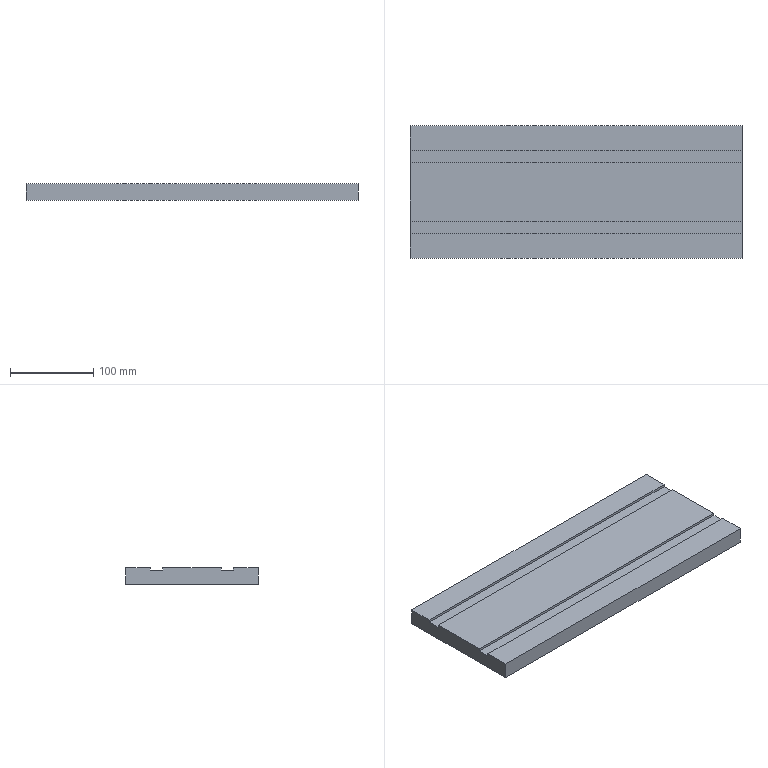Part | STEP file | Tube feed_id638_x_t | 1 solid | 14 faces | box 400 x 160 x 20 mm | volume 1244000 mm3 | plane 14
STEP:
#1=CARTESIAN_POINT('',(0.,0.,0.));
#2=DIRECTION('',(0.,0.,1.));
#3=DIRECTION('',(1.,0.,0.));
#4=AXIS2_PLACEMENT_3D('',#1,#2,#3);
#5=CARTESIAN_POINT('',(66.,461.936,-199.));
#6=VERTEX_POINT('',#5);
#7=CARTESIAN_POINT('',(66.,461.936,-202.));
#8=VERTEX_POINT('',#7);
#9=CARTESIAN_POINT('',(66.,461.936,-199.819));
#10=DIRECTION('',(0.,0.,-1.));
#11=VECTOR('',#10,1.);
#12=LINE('',#9,#11);
#13=CARTESIAN_POINT('',(66.,491.936,-199.));
#14=DIRECTION('',(1.,0.,0.));
#15=DIRECTION('',(0.,1.,0.));
#16=AXIS2_PLACEMENT_3D('',#13,#14,#15);
#17=PLANE('',#16);
#18=CARTESIAN_POINT('',(-30.,-0.8185));
#19=DIRECTION('',(0.,-1.));
#20=VECTOR('',#19,1.);
#21=LINE('',#18,#20);
#22=(GEOMETRIC_REPRESENTATION_CONTEXT(2)PARAMETRIC_REPRESENTATION_CONTEXT()REPRESENTATION_CONTEXT('',''));
#23=DEFINITIONAL_REPRESENTATION('',(#21),#22);
#24=PCURVE('',#17,#23);
#25=CARTESIAN_POINT('',(1137.73,461.936,-199.819));
#26=DIRECTION('',(0.,1.,0.));
#27=DIRECTION('',(0.,0.,1.));
#28=AXIS2_PLACEMENT_3D('',#25,#26,#27);
#29=PLANE('',#28);
#30=CARTESIAN_POINT('',(0.,-1071.73));
#31=DIRECTION('',(-1.,0.));
#32=VECTOR('',#31,1.);
#33=LINE('',#30,#32);
#34=(GEOMETRIC_REPRESENTATION_CONTEXT(2)PARAMETRIC_REPRESENTATION_CONTEXT()REPRESENTATION_CONTEXT('',''));
#35=DEFINITIONAL_REPRESENTATION('',(#33),#34);
#36=PCURVE('',#29,#35);
#37=SURFACE_CURVE('',#12,(#24,#36),.PCURVE_S1.);
#38=EDGE_CURVE('',#6,#8,#37,.T.);
#39=ORIENTED_EDGE('',*,*,#38,.F.);
#40=CARTESIAN_POINT('',(66.,491.936,-199.));
#41=VERTEX_POINT('',#40);
#42=CARTESIAN_POINT('',(66.,491.936,-199.));
#43=DIRECTION('',(0.,-1.,0.));
#44=VECTOR('',#43,1.);
#45=LINE('',#42,#44);
#46=CARTESIAN_POINT('',(0.,0.));
#47=DIRECTION('',(-1.,0.));
#48=VECTOR('',#47,1.);
#49=LINE('',#46,#48);
#50=(GEOMETRIC_REPRESENTATION_CONTEXT(2)PARAMETRIC_REPRESENTATION_CONTEXT()REPRESENTATION_CONTEXT('',''));
#51=DEFINITIONAL_REPRESENTATION('',(#49),#50);
#52=PCURVE('',#17,#51);
#53=CARTESIAN_POINT('',(0.,0.,-199.));
#54=DIRECTION('',(0.,0.,1.));
#55=DIRECTION('',(1.,0.,0.));
#56=AXIS2_PLACEMENT_3D('',#53,#54,#55);
#57=PLANE('',#56);
#58=CARTESIAN_POINT('',(66.,491.936));
#59=DIRECTION('',(0.,-1.));
#60=VECTOR('',#59,1.);
#61=LINE('',#58,#60);
#62=(GEOMETRIC_REPRESENTATION_CONTEXT(2)PARAMETRIC_REPRESENTATION_CONTEXT()REPRESENTATION_CONTEXT('',''));
#63=DEFINITIONAL_REPRESENTATION('',(#61),#62);
#64=PCURVE('',#57,#63);
#65=SURFACE_CURVE('',#45,(#52,#64),.PCURVE_S1.);
#66=EDGE_CURVE('',#41,#6,#65,.T.);
#67=ORIENTED_EDGE('',*,*,#66,.F.);
#68=CARTESIAN_POINT('',(66.,491.936,-219.));
#69=VERTEX_POINT('',#68);
#70=CARTESIAN_POINT('',(66.,491.936,-199.));
#71=DIRECTION('',(0.,0.,-1.));
#72=VECTOR('',#71,1.);
#73=LINE('',#70,#72);
#74=CARTESIAN_POINT('',(0.,0.));
#75=DIRECTION('',(0.,-1.));
#76=VECTOR('',#75,1.);
#77=LINE('',#74,#76);
#78=(GEOMETRIC_REPRESENTATION_CONTEXT(2)PARAMETRIC_REPRESENTATION_CONTEXT()REPRESENTATION_CONTEXT('',''));
#79=DEFINITIONAL_REPRESENTATION('',(#77),#78);
#80=PCURVE('',#17,#79);
#81=CARTESIAN_POINT('',(466.,491.936,-199.));
#82=DIRECTION('',(0.,-1.,0.));
#83=DIRECTION('',(0.,0.,-1.));
#84=AXIS2_PLACEMENT_3D('',#81,#82,#83);
#85=PLANE('',#84);
#86=CARTESIAN_POINT('',(0.,-400.));
#87=DIRECTION('',(1.,0.));
#88=VECTOR('',#87,1.);
#89=LINE('',#86,#88);
#90=(GEOMETRIC_REPRESENTATION_CONTEXT(2)PARAMETRIC_REPRESENTATION_CONTEXT()REPRESENTATION_CONTEXT('',''));
#91=DEFINITIONAL_REPRESENTATION('',(#89),#90);
#92=PCURVE('',#85,#91);
#93=SURFACE_CURVE('',#73,(#80,#92),.PCURVE_S1.);
#94=EDGE_CURVE('',#41,#69,#93,.T.);
#95=ORIENTED_EDGE('',*,*,#94,.T.);
#96=CARTESIAN_POINT('',(66.,331.936,-219.));
#97=VERTEX_POINT('',#96);
#98=CARTESIAN_POINT('',(66.,491.936,-219.));
#99=DIRECTION('',(0.,-1.,0.));
#100=VECTOR('',#99,1.);
#101=LINE('',#98,#100);
#102=CARTESIAN_POINT('',(0.,-20.));
#103=DIRECTION('',(-1.,0.));
#104=VECTOR('',#103,1.);
#105=LINE('',#102,#104);
#106=(GEOMETRIC_REPRESENTATION_CONTEXT(2)PARAMETRIC_REPRESENTATION_CONTEXT()REPRESENTATION_CONTEXT('',''));
#107=DEFINITIONAL_REPRESENTATION('',(#105),#106);
#108=PCURVE('',#17,#107);
#109=CARTESIAN_POINT('',(0.,0.,-219.));
#110=DIRECTION('',(0.,0.,1.));
#111=DIRECTION('',(1.,0.,0.));
#112=AXIS2_PLACEMENT_3D('',#109,#110,#111);
#113=PLANE('',#112);
#114=CARTESIAN_POINT('',(66.,491.936));
#115=DIRECTION('',(0.,-1.));
#116=VECTOR('',#115,1.);
#117=LINE('',#114,#116);
#118=(GEOMETRIC_REPRESENTATION_CONTEXT(2)PARAMETRIC_REPRESENTATION_CONTEXT()REPRESENTATION_CONTEXT('',''));
#119=DEFINITIONAL_REPRESENTATION('',(#117),#118);
#120=PCURVE('',#113,#119);
#121=SURFACE_CURVE('',#101,(#108,#120),.PCURVE_S1.);
#122=EDGE_CURVE('',#69,#97,#121,.T.);
#123=ORIENTED_EDGE('',*,*,#122,.T.);
#124=CARTESIAN_POINT('',(66.,331.936,-199.));
#125=VERTEX_POINT('',#124);
#126=CARTESIAN_POINT('',(66.,331.936,-199.));
#127=DIRECTION('',(0.,0.,-1.));
#128=VECTOR('',#127,1.);
#129=LINE('',#126,#128);
#130=CARTESIAN_POINT('',(-160.,0.));
#131=DIRECTION('',(0.,-1.));
#132=VECTOR('',#131,1.);
#133=LINE('',#130,#132);
#134=(GEOMETRIC_REPRESENTATION_CONTEXT(2)PARAMETRIC_REPRESENTATION_CONTEXT()REPRESENTATION_CONTEXT('',''));
#135=DEFINITIONAL_REPRESENTATION('',(#133),#134);
#136=PCURVE('',#17,#135);
#137=CARTESIAN_POINT('',(66.,331.936,-199.));
#138=DIRECTION('',(0.,1.,0.));
#139=DIRECTION('',(-1.,0.,0.));
#140=AXIS2_PLACEMENT_3D('',#137,#138,#139);
#141=PLANE('',#140);
#142=CARTESIAN_POINT('',(0.,0.));
#143=DIRECTION('',(0.,-1.));
#144=VECTOR('',#143,1.);
#145=LINE('',#142,#144);
#146=(GEOMETRIC_REPRESENTATION_CONTEXT(2)PARAMETRIC_REPRESENTATION_CONTEXT()REPRESENTATION_CONTEXT('',''));
#147=DEFINITIONAL_REPRESENTATION('',(#145),#146);
#148=PCURVE('',#141,#147);
#149=SURFACE_CURVE('',#129,(#136,#148),.PCURVE_S1.);
#150=EDGE_CURVE('',#125,#97,#149,.T.);
#151=ORIENTED_EDGE('',*,*,#150,.F.);
#152=CARTESIAN_POINT('',(66.,361.936,-199.));
#153=VERTEX_POINT('',#152);
#154=CARTESIAN_POINT('',(66.,491.936,-199.));
#155=DIRECTION('',(0.,-1.,0.));
#156=VECTOR('',#155,1.);
#157=LINE('',#154,#156);
#158=CARTESIAN_POINT('',(0.,0.));
#159=DIRECTION('',(-1.,0.));
#160=VECTOR('',#159,1.);
#161=LINE('',#158,#160);
#162=(GEOMETRIC_REPRESENTATION_CONTEXT(2)PARAMETRIC_REPRESENTATION_CONTEXT()REPRESENTATION_CONTEXT('',''));
#163=DEFINITIONAL_REPRESENTATION('',(#161),#162);
#164=PCURVE('',#17,#163);
#165=CARTESIAN_POINT('',(0.,0.,-199.));
#166=DIRECTION('',(0.,0.,1.));
#167=DIRECTION('',(1.,0.,0.));
#168=AXIS2_PLACEMENT_3D('',#165,#166,#167);
#169=PLANE('',#168);
#170=CARTESIAN_POINT('',(66.,491.936));
#171=DIRECTION('',(0.,-1.));
#172=VECTOR('',#171,1.);
#173=LINE('',#170,#172);
#174=(GEOMETRIC_REPRESENTATION_CONTEXT(2)PARAMETRIC_REPRESENTATION_CONTEXT()REPRESENTATION_CONTEXT('',''));
#175=DEFINITIONAL_REPRESENTATION('',(#173),#174);
#176=PCURVE('',#169,#175);
#177=SURFACE_CURVE('',#157,(#164,#176),.PCURVE_S1.);
#178=EDGE_CURVE('',#153,#125,#177,.T.);
#179=ORIENTED_EDGE('',*,*,#178,.F.);
#180=CARTESIAN_POINT('',(66.,361.936,-202.));
#181=VERTEX_POINT('',#180);
#182=CARTESIAN_POINT('',(66.,361.936,-201.));
#183=DIRECTION('',(0.,0.,1.));
#184=VECTOR('',#183,1.);
#185=LINE('',#182,#184);
#186=CARTESIAN_POINT('',(-130.,-2.));
#187=DIRECTION('',(0.,1.));
#188=VECTOR('',#187,1.);
#189=LINE('',#186,#188);
#190=(GEOMETRIC_REPRESENTATION_CONTEXT(2)PARAMETRIC_REPRESENTATION_CONTEXT()REPRESENTATION_CONTEXT('',''));
#191=DEFINITIONAL_REPRESENTATION('',(#189),#190);
#192=PCURVE('',#17,#191);
#193=CARTESIAN_POINT('',(1137.73,361.936,-201.));
#194=DIRECTION('',(0.,-1.,0.));
#195=DIRECTION('',(0.,0.,-1.));
#196=AXIS2_PLACEMENT_3D('',#193,#194,#195);
#197=PLANE('',#196);
#198=CARTESIAN_POINT('',(0.,-1071.73));
#199=DIRECTION('',(-1.,0.));
#200=VECTOR('',#199,1.);
#201=LINE('',#198,#200);
#202=(GEOMETRIC_REPRESENTATION_CONTEXT(2)PARAMETRIC_REPRESENTATION_CONTEXT()REPRESENTATION_CONTEXT('',''));
#203=DEFINITIONAL_REPRESENTATION('',(#201),#202);
#204=PCURVE('',#197,#203);
#205=SURFACE_CURVE('',#185,(#192,#204),.PCURVE_S1.);
#206=EDGE_CURVE('',#181,#153,#205,.T.);
#207=ORIENTED_EDGE('',*,*,#206,.F.);
#208=CARTESIAN_POINT('',(66.,376.936,-202.));
#209=VERTEX_POINT('',#208);
#210=CARTESIAN_POINT('',(66.,376.936,-202.));
#211=DIRECTION('',(0.,-1.,0.));
#212=VECTOR('',#211,1.);
#213=LINE('',#210,#212);
#214=CARTESIAN_POINT('',(-115.,-3.));
#215=DIRECTION('',(-1.,0.));
#216=VECTOR('',#215,1.);
#217=LINE('',#214,#216);
#218=(GEOMETRIC_REPRESENTATION_CONTEXT(2)PARAMETRIC_REPRESENTATION_CONTEXT()REPRESENTATION_CONTEXT('',''));
#219=DEFINITIONAL_REPRESENTATION('',(#217),#218);
#220=PCURVE('',#17,#219);
#221=CARTESIAN_POINT('',(1137.73,376.936,-202.));
#222=DIRECTION('',(0.,0.,-1.));
#223=DIRECTION('',(-1.,0.,0.));
#224=AXIS2_PLACEMENT_3D('',#221,#222,#223);
#225=PLANE('',#224);
#226=CARTESIAN_POINT('',(1071.73,0.));
#227=DIRECTION('',(0.,-1.));
#228=VECTOR('',#227,1.);
#229=LINE('',#226,#228);
#230=(GEOMETRIC_REPRESENTATION_CONTEXT(2)PARAMETRIC_REPRESENTATION_CONTEXT()REPRESENTATION_CONTEXT('',''));
#231=DEFINITIONAL_REPRESENTATION('',(#229),#230);
#232=PCURVE('',#225,#231);
#233=SURFACE_CURVE('',#213,(#220,#232),.PCURVE_S1.);
#234=EDGE_CURVE('',#209,#181,#233,.T.);
#235=ORIENTED_EDGE('',*,*,#234,.F.);
#236=CARTESIAN_POINT('',(66.,376.936,-199.));
#237=VERTEX_POINT('',#236);
#238=CARTESIAN_POINT('',(66.,376.936,-199.819));
#239=DIRECTION('',(0.,0.,-1.));
#240=VECTOR('',#239,1.);
#241=LINE('',#238,#240);
#242=CARTESIAN_POINT('',(-115.,-0.8185));
#243=DIRECTION('',(0.,-1.));
#244=VECTOR('',#243,1.);
#245=LINE('',#242,#244);
#246=(GEOMETRIC_REPRESENTATION_CONTEXT(2)PARAMETRIC_REPRESENTATION_CONTEXT()REPRESENTATION_CONTEXT('',''));
#247=DEFINITIONAL_REPRESENTATION('',(#245),#246);
#248=PCURVE('',#17,#247);
#249=CARTESIAN_POINT('',(1137.73,376.936,-199.819));
#250=DIRECTION('',(0.,1.,0.));
#251=DIRECTION('',(0.,0.,1.));
#252=AXIS2_PLACEMENT_3D('',#249,#250,#251);
#253=PLANE('',#252);
#254=CARTESIAN_POINT('',(0.,-1071.73));
#255=DIRECTION('',(-1.,0.));
#256=VECTOR('',#255,1.);
#257=LINE('',#254,#256);
#258=(GEOMETRIC_REPRESENTATION_CONTEXT(2)PARAMETRIC_REPRESENTATION_CONTEXT()REPRESENTATION_CONTEXT('',''));
#259=DEFINITIONAL_REPRESENTATION('',(#257),#258);
#260=PCURVE('',#253,#259);
#261=SURFACE_CURVE('',#241,(#248,#260),.PCURVE_S1.);
#262=EDGE_CURVE('',#237,#209,#261,.T.);
#263=ORIENTED_EDGE('',*,*,#262,.F.);
#264=CARTESIAN_POINT('',(66.,446.936,-199.));
#265=VERTEX_POINT('',#264);
#266=CARTESIAN_POINT('',(66.,491.936,-199.));
#267=DIRECTION('',(0.,-1.,0.));
#268=VECTOR('',#267,1.);
#269=LINE('',#266,#268);
#270=CARTESIAN_POINT('',(0.,0.));
#271=DIRECTION('',(-1.,0.));
#272=VECTOR('',#271,1.);
#273=LINE('',#270,#272);
#274=(GEOMETRIC_REPRESENTATION_CONTEXT(2)PARAMETRIC_REPRESENTATION_CONTEXT()REPRESENTATION_CONTEXT('',''));
#275=DEFINITIONAL_REPRESENTATION('',(#273),#274);
#276=PCURVE('',#17,#275);
#277=CARTESIAN_POINT('',(0.,0.,-199.));
#278=DIRECTION('',(0.,0.,1.));
#279=DIRECTION('',(1.,0.,0.));
#280=AXIS2_PLACEMENT_3D('',#277,#278,#279);
#281=PLANE('',#280);
#282=CARTESIAN_POINT('',(66.,491.936));
#283=DIRECTION('',(0.,-1.));
#284=VECTOR('',#283,1.);
#285=LINE('',#282,#284);
#286=(GEOMETRIC_REPRESENTATION_CONTEXT(2)PARAMETRIC_REPRESENTATION_CONTEXT()REPRESENTATION_CONTEXT('',''));
#287=DEFINITIONAL_REPRESENTATION('',(#285),#286);
#288=PCURVE('',#281,#287);
#289=SURFACE_CURVE('',#269,(#276,#288),.PCURVE_S1.);
#290=EDGE_CURVE('',#265,#237,#289,.T.);
#291=ORIENTED_EDGE('',*,*,#290,.F.);
#292=CARTESIAN_POINT('',(66.,446.936,-202.));
#293=VERTEX_POINT('',#292);
#294=CARTESIAN_POINT('',(66.,446.936,-201.));
#295=DIRECTION('',(0.,0.,1.));
#296=VECTOR('',#295,1.);
#297=LINE('',#294,#296);
#298=CARTESIAN_POINT('',(-45.,-2.));
#299=DIRECTION('',(0.,1.));
#300=VECTOR('',#299,1.);
#301=LINE('',#298,#300);
#302=(GEOMETRIC_REPRESENTATION_CONTEXT(2)PARAMETRIC_REPRESENTATION_CONTEXT()REPRESENTATION_CONTEXT('',''));
#303=DEFINITIONAL_REPRESENTATION('',(#301),#302);
#304=PCURVE('',#17,#303);
#305=CARTESIAN_POINT('',(1137.73,446.936,-201.));
#306=DIRECTION('',(0.,-1.,0.));
#307=DIRECTION('',(0.,0.,-1.));
#308=AXIS2_PLACEMENT_3D('',#305,#306,#307);
#309=PLANE('',#308);
#310=CARTESIAN_POINT('',(0.,-1071.73));
#311=DIRECTION('',(-1.,0.));
#312=VECTOR('',#311,1.);
#313=LINE('',#310,#312);
#314=(GEOMETRIC_REPRESENTATION_CONTEXT(2)PARAMETRIC_REPRESENTATION_CONTEXT()REPRESENTATION_CONTEXT('',''));
#315=DEFINITIONAL_REPRESENTATION('',(#313),#314);
#316=PCURVE('',#309,#315);
#317=SURFACE_CURVE('',#297,(#304,#316),.PCURVE_S1.);
#318=EDGE_CURVE('',#293,#265,#317,.T.);
#319=ORIENTED_EDGE('',*,*,#318,.F.);
#320=CARTESIAN_POINT('',(66.,461.936,-202.));
#321=DIRECTION('',(0.,-1.,0.));
#322=VECTOR('',#321,1.);
#323=LINE('',#320,#322);
#324=CARTESIAN_POINT('',(-30.,-3.));
#325=DIRECTION('',(-1.,0.));
#326=VECTOR('',#325,1.);
#327=LINE('',#324,#326);
#328=(GEOMETRIC_REPRESENTATION_CONTEXT(2)PARAMETRIC_REPRESENTATION_CONTEXT()REPRESENTATION_CONTEXT('',''));
#329=DEFINITIONAL_REPRESENTATION('',(#327),#328);
#330=PCURVE('',#17,#329);
#331=CARTESIAN_POINT('',(1137.73,461.936,-202.));
#332=DIRECTION('',(0.,0.,-1.));
#333=DIRECTION('',(-1.,0.,0.));
#334=AXIS2_PLACEMENT_3D('',#331,#332,#333);
#335=PLANE('',#334);
#336=CARTESIAN_POINT('',(1071.73,0.));
#337=DIRECTION('',(0.,-1.));
#338=VECTOR('',#337,1.);
#339=LINE('',#336,#338);
#340=(GEOMETRIC_REPRESENTATION_CONTEXT(2)PARAMETRIC_REPRESENTATION_CONTEXT()REPRESENTATION_CONTEXT('',''));
#341=DEFINITIONAL_REPRESENTATION('',(#339),#340);
#342=PCURVE('',#335,#341);
#343=SURFACE_CURVE('',#323,(#330,#342),.PCURVE_S1.);
#344=EDGE_CURVE('',#8,#293,#343,.T.);
#345=ORIENTED_EDGE('',*,*,#344,.F.);
#346=EDGE_LOOP('',(#39,#67,#95,#123,#151,#179,#207,#235,#263,#291,#319,#345));
#347=FACE_BOUND('',#346,.T.);
#348=ADVANCED_FACE('',(#347),#17,.F.);
#349=CARTESIAN_POINT('',(466.,446.936,-199.));
#350=VERTEX_POINT('',#349);
#351=CARTESIAN_POINT('',(466.,446.936,-202.));
#352=VERTEX_POINT('',#351);
#353=CARTESIAN_POINT('',(466.,446.936,-201.));
#354=DIRECTION('',(0.,0.,-1.));
#355=VECTOR('',#354,1.);
#356=LINE('',#353,#355);
#357=CARTESIAN_POINT('',(466.,331.936,-199.));
#358=DIRECTION('',(-1.,0.,0.));
#359=DIRECTION('',(0.,0.,1.));
#360=AXIS2_PLACEMENT_3D('',#357,#358,#359);
#361=PLANE('',#360);
#362=CARTESIAN_POINT('',(-2.,115.));
#363=DIRECTION('',(-1.,0.));
#364=VECTOR('',#363,1.);
#365=LINE('',#362,#364);
#366=(GEOMETRIC_REPRESENTATION_CONTEXT(2)PARAMETRIC_REPRESENTATION_CONTEXT()REPRESENTATION_CONTEXT('',''));
#367=DEFINITIONAL_REPRESENTATION('',(#365),#366);
#368=PCURVE('',#361,#367);
#369=CARTESIAN_POINT('',(0.,-671.73));
#370=DIRECTION('',(1.,0.));
#371=VECTOR('',#370,1.);
#372=LINE('',#369,#371);
#373=(GEOMETRIC_REPRESENTATION_CONTEXT(2)PARAMETRIC_REPRESENTATION_CONTEXT()REPRESENTATION_CONTEXT('',''));
#374=DEFINITIONAL_REPRESENTATION('',(#372),#373);
#375=PCURVE('',#309,#374);
#376=SURFACE_CURVE('',#356,(#368,#375),.PCURVE_S1.);
#377=EDGE_CURVE('',#350,#352,#376,.T.);
#378=ORIENTED_EDGE('',*,*,#377,.F.);
#379=CARTESIAN_POINT('',(466.,376.936,-199.));
#380=VERTEX_POINT('',#379);
#381=CARTESIAN_POINT('',(466.,331.936,-199.));
#382=DIRECTION('',(0.,1.,0.));
#383=VECTOR('',#382,1.);
#384=LINE('',#381,#383);
#385=CARTESIAN_POINT('',(0.,0.));
#386=DIRECTION('',(0.,1.));
#387=VECTOR('',#386,1.);
#388=LINE('',#385,#387);
#389=(GEOMETRIC_REPRESENTATION_CONTEXT(2)PARAMETRIC_REPRESENTATION_CONTEXT()REPRESENTATION_CONTEXT('',''));
#390=DEFINITIONAL_REPRESENTATION('',(#388),#389);
#391=PCURVE('',#361,#390);
#392=CARTESIAN_POINT('',(466.,331.936));
#393=DIRECTION('',(0.,1.));
#394=VECTOR('',#393,1.);
#395=LINE('',#392,#394);
#396=(GEOMETRIC_REPRESENTATION_CONTEXT(2)PARAMETRIC_REPRESENTATION_CONTEXT()REPRESENTATION_CONTEXT('',''));
#397=DEFINITIONAL_REPRESENTATION('',(#395),#396);
#398=PCURVE('',#281,#397);
#399=SURFACE_CURVE('',#384,(#391,#398),.PCURVE_S1.);
#400=EDGE_CURVE('',#380,#350,#399,.T.);
#401=ORIENTED_EDGE('',*,*,#400,.F.);
#402=CARTESIAN_POINT('',(466.,376.936,-202.));
#403=VERTEX_POINT('',#402);
#404=CARTESIAN_POINT('',(466.,376.936,-199.819));
#405=DIRECTION('',(0.,0.,1.));
#406=VECTOR('',#405,1.);
#407=LINE('',#404,#406);
#408=CARTESIAN_POINT('',(-0.8185,45.));
#409=DIRECTION('',(1.,0.));
#410=VECTOR('',#409,1.);
#411=LINE('',#408,#410);
#412=(GEOMETRIC_REPRESENTATION_CONTEXT(2)PARAMETRIC_REPRESENTATION_CONTEXT()REPRESENTATION_CONTEXT('',''));
#413=DEFINITIONAL_REPRESENTATION('',(#411),#412);
#414=PCURVE('',#361,#413);
#415=CARTESIAN_POINT('',(0.,-671.73));
#416=DIRECTION('',(1.,0.));
#417=VECTOR('',#416,1.);
#418=LINE('',#415,#417);
#419=(GEOMETRIC_REPRESENTATION_CONTEXT(2)PARAMETRIC_REPRESENTATION_CONTEXT()REPRESENTATION_CONTEXT('',''));
#420=DEFINITIONAL_REPRESENTATION('',(#418),#419);
#421=PCURVE('',#253,#420);
#422=SURFACE_CURVE('',#407,(#414,#421),.PCURVE_S1.);
#423=EDGE_CURVE('',#403,#380,#422,.T.);
#424=ORIENTED_EDGE('',*,*,#423,.F.);
#425=CARTESIAN_POINT('',(466.,361.936,-202.));
#426=VERTEX_POINT('',#425);
#427=CARTESIAN_POINT('',(466.,376.936,-202.));
#428=DIRECTION('',(0.,1.,0.));
#429=VECTOR('',#428,1.);
#430=LINE('',#427,#429);
#431=CARTESIAN_POINT('',(-3.,45.));
#432=DIRECTION('',(0.,1.));
#433=VECTOR('',#432,1.);
#434=LINE('',#431,#433);
#435=(GEOMETRIC_REPRESENTATION_CONTEXT(2)PARAMETRIC_REPRESENTATION_CONTEXT()REPRESENTATION_CONTEXT('',''));
#436=DEFINITIONAL_REPRESENTATION('',(#434),#435);
#437=PCURVE('',#361,#436);
#438=CARTESIAN_POINT('',(671.73,0.));
#439=DIRECTION('',(0.,1.));
#440=VECTOR('',#439,1.);
#441=LINE('',#438,#440);
#442=(GEOMETRIC_REPRESENTATION_CONTEXT(2)PARAMETRIC_REPRESENTATION_CONTEXT()REPRESENTATION_CONTEXT('',''));
#443=DEFINITIONAL_REPRESENTATION('',(#441),#442);
#444=PCURVE('',#225,#443);
#445=SURFACE_CURVE('',#430,(#437,#444),.PCURVE_S1.);
#446=EDGE_CURVE('',#426,#403,#445,.T.);
#447=ORIENTED_EDGE('',*,*,#446,.F.);
#448=CARTESIAN_POINT('',(466.,361.936,-199.));
#449=VERTEX_POINT('',#448);
#450=CARTESIAN_POINT('',(466.,361.936,-201.));
#451=DIRECTION('',(0.,0.,-1.));
#452=VECTOR('',#451,1.);
#453=LINE('',#450,#452);
#454=CARTESIAN_POINT('',(-2.,30.));
#455=DIRECTION('',(-1.,0.));
#456=VECTOR('',#455,1.);
#457=LINE('',#454,#456);
#458=(GEOMETRIC_REPRESENTATION_CONTEXT(2)PARAMETRIC_REPRESENTATION_CONTEXT()REPRESENTATION_CONTEXT('',''));
#459=DEFINITIONAL_REPRESENTATION('',(#457),#458);
#460=PCURVE('',#361,#459);
#461=CARTESIAN_POINT('',(0.,-671.73));
#462=DIRECTION('',(1.,0.));
#463=VECTOR('',#462,1.);
#464=LINE('',#461,#463);
#465=(GEOMETRIC_REPRESENTATION_CONTEXT(2)PARAMETRIC_REPRESENTATION_CONTEXT()REPRESENTATION_CONTEXT('',''));
#466=DEFINITIONAL_REPRESENTATION('',(#464),#465);
#467=PCURVE('',#197,#466);
#468=SURFACE_CURVE('',#453,(#460,#467),.PCURVE_S1.);
#469=EDGE_CURVE('',#449,#426,#468,.T.);
#470=ORIENTED_EDGE('',*,*,#469,.F.);
#471=CARTESIAN_POINT('',(466.,331.936,-199.));
#472=VERTEX_POINT('',#471);
#473=CARTESIAN_POINT('',(466.,331.936,-199.));
#474=DIRECTION('',(0.,1.,0.));
#475=VECTOR('',#474,1.);
#476=LINE('',#473,#475);
#477=CARTESIAN_POINT('',(0.,0.));
#478=DIRECTION('',(0.,1.));
#479=VECTOR('',#478,1.);
#480=LINE('',#477,#479);
#481=(GEOMETRIC_REPRESENTATION_CONTEXT(2)PARAMETRIC_REPRESENTATION_CONTEXT()REPRESENTATION_CONTEXT('',''));
#482=DEFINITIONAL_REPRESENTATION('',(#480),#481);
#483=PCURVE('',#361,#482);
#484=CARTESIAN_POINT('',(466.,331.936));
#485=DIRECTION('',(0.,1.));
#486=VECTOR('',#485,1.);
#487=LINE('',#484,#486);
#488=(GEOMETRIC_REPRESENTATION_CONTEXT(2)PARAMETRIC_REPRESENTATION_CONTEXT()REPRESENTATION_CONTEXT('',''));
#489=DEFINITIONAL_REPRESENTATION('',(#487),#488);
#490=PCURVE('',#169,#489);
#491=SURFACE_CURVE('',#476,(#483,#490),.PCURVE_S1.);
#492=EDGE_CURVE('',#472,#449,#491,.T.);
#493=ORIENTED_EDGE('',*,*,#492,.F.);
#494=CARTESIAN_POINT('',(466.,331.936,-219.));
#495=VERTEX_POINT('',#494);
#496=CARTESIAN_POINT('',(466.,331.936,-199.));
#497=DIRECTION('',(0.,0.,-1.));
#498=VECTOR('',#497,1.);
#499=LINE('',#496,#498);
#500=CARTESIAN_POINT('',(0.,0.));
#501=DIRECTION('',(-1.,0.));
#502=VECTOR('',#501,1.);
#503=LINE('',#500,#502);
#504=(GEOMETRIC_REPRESENTATION_CONTEXT(2)PARAMETRIC_REPRESENTATION_CONTEXT()REPRESENTATION_CONTEXT('',''));
#505=DEFINITIONAL_REPRESENTATION('',(#503),#504);
#506=PCURVE('',#361,#505);
#507=CARTESIAN_POINT('',(-400.,0.));
#508=DIRECTION('',(0.,-1.));
#509=VECTOR('',#508,1.);
#510=LINE('',#507,#509);
#511=(GEOMETRIC_REPRESENTATION_CONTEXT(2)PARAMETRIC_REPRESENTATION_CONTEXT()REPRESENTATION_CONTEXT('',''));
#512=DEFINITIONAL_REPRESENTATION('',(#510),#511);
#513=PCURVE('',#141,#512);
#514=SURFACE_CURVE('',#499,(#506,#513),.PCURVE_S1.);
#515=EDGE_CURVE('',#472,#495,#514,.T.);
#516=ORIENTED_EDGE('',*,*,#515,.T.);
#517=CARTESIAN_POINT('',(466.,491.936,-219.));
#518=VERTEX_POINT('',#517);
#519=CARTESIAN_POINT('',(466.,331.936,-219.));
#520=DIRECTION('',(0.,1.,0.));
#521=VECTOR('',#520,1.);
#522=LINE('',#519,#521);
#523=CARTESIAN_POINT('',(-20.,0.));
#524=DIRECTION('',(0.,1.));
#525=VECTOR('',#524,1.);
#526=LINE('',#523,#525);
#527=(GEOMETRIC_REPRESENTATION_CONTEXT(2)PARAMETRIC_REPRESENTATION_CONTEXT()REPRESENTATION_CONTEXT('',''));
#528=DEFINITIONAL_REPRESENTATION('',(#526),#527);
#529=PCURVE('',#361,#528);
#530=CARTESIAN_POINT('',(466.,331.936));
#531=DIRECTION('',(0.,1.));
#532=VECTOR('',#531,1.);
#533=LINE('',#530,#532);
#534=(GEOMETRIC_REPRESENTATION_CONTEXT(2)PARAMETRIC_REPRESENTATION_CONTEXT()REPRESENTATION_CONTEXT('',''));
#535=DEFINITIONAL_REPRESENTATION('',(#533),#534);
#536=PCURVE('',#113,#535);
#537=SURFACE_CURVE('',#522,(#529,#536),.PCURVE_S1.);
#538=EDGE_CURVE('',#495,#518,#537,.T.);
#539=ORIENTED_EDGE('',*,*,#538,.T.);
#540=CARTESIAN_POINT('',(466.,491.936,-199.));
#541=VERTEX_POINT('',#540);
#542=CARTESIAN_POINT('',(466.,491.936,-199.));
#543=DIRECTION('',(0.,0.,-1.));
#544=VECTOR('',#543,1.);
#545=LINE('',#542,#544);
#546=CARTESIAN_POINT('',(0.,160.));
#547=DIRECTION('',(-1.,0.));
#548=VECTOR('',#547,1.);
#549=LINE('',#546,#548);
#550=(GEOMETRIC_REPRESENTATION_CONTEXT(2)PARAMETRIC_REPRESENTATION_CONTEXT()REPRESENTATION_CONTEXT('',''));
#551=DEFINITIONAL_REPRESENTATION('',(#549),#550);
#552=PCURVE('',#361,#551);
#553=CARTESIAN_POINT('',(0.,0.));
#554=DIRECTION('',(1.,0.));
#555=VECTOR('',#554,1.);
#556=LINE('',#553,#555);
#557=(GEOMETRIC_REPRESENTATION_CONTEXT(2)PARAMETRIC_REPRESENTATION_CONTEXT()REPRESENTATION_CONTEXT('',''));
#558=DEFINITIONAL_REPRESENTATION('',(#556),#557);
#559=PCURVE('',#85,#558);
#560=SURFACE_CURVE('',#545,(#552,#559),.PCURVE_S1.);
#561=EDGE_CURVE('',#541,#518,#560,.T.);
#562=ORIENTED_EDGE('',*,*,#561,.F.);
#563=CARTESIAN_POINT('',(466.,461.936,-199.));
#564=VERTEX_POINT('',#563);
#565=CARTESIAN_POINT('',(466.,331.936,-199.));
#566=DIRECTION('',(0.,1.,0.));
#567=VECTOR('',#566,1.);
#568=LINE('',#565,#567);
#569=CARTESIAN_POINT('',(0.,0.));
#570=DIRECTION('',(0.,1.));
#571=VECTOR('',#570,1.);
#572=LINE('',#569,#571);
#573=(GEOMETRIC_REPRESENTATION_CONTEXT(2)PARAMETRIC_REPRESENTATION_CONTEXT()REPRESENTATION_CONTEXT('',''));
#574=DEFINITIONAL_REPRESENTATION('',(#572),#573);
#575=PCURVE('',#361,#574);
#576=CARTESIAN_POINT('',(466.,331.936));
#577=DIRECTION('',(0.,1.));
#578=VECTOR('',#577,1.);
#579=LINE('',#576,#578);
#580=(GEOMETRIC_REPRESENTATION_CONTEXT(2)PARAMETRIC_REPRESENTATION_CONTEXT()REPRESENTATION_CONTEXT('',''));
#581=DEFINITIONAL_REPRESENTATION('',(#579),#580);
#582=PCURVE('',#57,#581);
#583=SURFACE_CURVE('',#568,(#575,#582),.PCURVE_S1.);
#584=EDGE_CURVE('',#564,#541,#583,.T.);
#585=ORIENTED_EDGE('',*,*,#584,.F.);
#586=CARTESIAN_POINT('',(466.,461.936,-202.));
#587=VERTEX_POINT('',#586);
#588=CARTESIAN_POINT('',(466.,461.936,-199.819));
#589=DIRECTION('',(0.,0.,1.));
#590=VECTOR('',#589,1.);
#591=LINE('',#588,#590);
#592=CARTESIAN_POINT('',(-0.8185,130.));
#593=DIRECTION('',(1.,0.));
#594=VECTOR('',#593,1.);
#595=LINE('',#592,#594);
#596=(GEOMETRIC_REPRESENTATION_CONTEXT(2)PARAMETRIC_REPRESENTATION_CONTEXT()REPRESENTATION_CONTEXT('',''));
#597=DEFINITIONAL_REPRESENTATION('',(#595),#596);
#598=PCURVE('',#361,#597);
#599=CARTESIAN_POINT('',(0.,-671.73));
#600=DIRECTION('',(1.,0.));
#601=VECTOR('',#600,1.);
#602=LINE('',#599,#601);
#603=(GEOMETRIC_REPRESENTATION_CONTEXT(2)PARAMETRIC_REPRESENTATION_CONTEXT()REPRESENTATION_CONTEXT('',''));
#604=DEFINITIONAL_REPRESENTATION('',(#602),#603);
#605=PCURVE('',#29,#604);
#606=SURFACE_CURVE('',#591,(#598,#605),.PCURVE_S1.);
#607=EDGE_CURVE('',#587,#564,#606,.T.);
#608=ORIENTED_EDGE('',*,*,#607,.F.);
#609=CARTESIAN_POINT('',(466.,461.936,-202.));
#610=DIRECTION('',(0.,1.,0.));
#611=VECTOR('',#610,1.);
#612=LINE('',#609,#611);
#613=CARTESIAN_POINT('',(-3.,130.));
#614=DIRECTION('',(0.,1.));
#615=VECTOR('',#614,1.);
#616=LINE('',#613,#615);
#617=(GEOMETRIC_REPRESENTATION_CONTEXT(2)PARAMETRIC_REPRESENTATION_CONTEXT()REPRESENTATION_CONTEXT('',''));
#618=DEFINITIONAL_REPRESENTATION('',(#616),#617);
#619=PCURVE('',#361,#618);
#620=CARTESIAN_POINT('',(671.73,0.));
#621=DIRECTION('',(0.,1.));
#622=VECTOR('',#621,1.);
#623=LINE('',#620,#622);
#624=(GEOMETRIC_REPRESENTATION_CONTEXT(2)PARAMETRIC_REPRESENTATION_CONTEXT()REPRESENTATION_CONTEXT('',''));
#625=DEFINITIONAL_REPRESENTATION('',(#623),#624);
#626=PCURVE('',#335,#625);
#627=SURFACE_CURVE('',#612,(#619,#626),.PCURVE_S1.);
#628=EDGE_CURVE('',#352,#587,#627,.T.);
#629=ORIENTED_EDGE('',*,*,#628,.F.);
#630=EDGE_LOOP('',(#378,#401,#424,#447,#470,#493,#516,#539,#562,#585,#608,#629));
#631=FACE_BOUND('',#630,.T.);
#632=ADVANCED_FACE('',(#631),#361,.F.);
#633=CARTESIAN_POINT('',(0.,446.936,-199.));
#634=DIRECTION('',(1.,0.,0.));
#635=VECTOR('',#634,1.);
#636=LINE('',#633,#635);
#637=CARTESIAN_POINT('',(0.,446.936));
#638=DIRECTION('',(1.,0.));
#639=VECTOR('',#638,1.);
#640=LINE('',#637,#639);
#641=(GEOMETRIC_REPRESENTATION_CONTEXT(2)PARAMETRIC_REPRESENTATION_CONTEXT()REPRESENTATION_CONTEXT('',''));
#642=DEFINITIONAL_REPRESENTATION('',(#640),#641);
#643=PCURVE('',#281,#642);
#644=CARTESIAN_POINT('',(-2.,-1137.73));
#645=DIRECTION('',(0.,1.));
#646=VECTOR('',#645,1.);
#647=LINE('',#644,#646);
#648=(GEOMETRIC_REPRESENTATION_CONTEXT(2)PARAMETRIC_REPRESENTATION_CONTEXT()REPRESENTATION_CONTEXT('',''));
#649=DEFINITIONAL_REPRESENTATION('',(#647),#648);
#650=PCURVE('',#309,#649);
#651=SURFACE_CURVE('',#636,(#643,#650),.PCURVE_S1.);
#652=EDGE_CURVE('',#265,#350,#651,.T.);
#653=ORIENTED_EDGE('',*,*,#652,.F.);
#654=ORIENTED_EDGE('',*,*,#290,.T.);
#655=CARTESIAN_POINT('',(0.,376.936,-199.));
#656=DIRECTION('',(-1.,0.,0.));
#657=VECTOR('',#656,1.);
#658=LINE('',#655,#657);
#659=CARTESIAN_POINT('',(0.,376.936));
#660=DIRECTION('',(-1.,0.));
#661=VECTOR('',#660,1.);
#662=LINE('',#659,#661);
#663=(GEOMETRIC_REPRESENTATION_CONTEXT(2)PARAMETRIC_REPRESENTATION_CONTEXT()REPRESENTATION_CONTEXT('',''));
#664=DEFINITIONAL_REPRESENTATION('',(#662),#663);
#665=PCURVE('',#281,#664);
#666=CARTESIAN_POINT('',(0.8185,-1137.73));
#667=DIRECTION('',(0.,-1.));
#668=VECTOR('',#667,1.);
#669=LINE('',#666,#668);
#670=(GEOMETRIC_REPRESENTATION_CONTEXT(2)PARAMETRIC_REPRESENTATION_CONTEXT()REPRESENTATION_CONTEXT('',''));
#671=DEFINITIONAL_REPRESENTATION('',(#669),#670);
#672=PCURVE('',#253,#671);
#673=SURFACE_CURVE('',#658,(#665,#672),.PCURVE_S1.);
#674=EDGE_CURVE('',#380,#237,#673,.T.);
#675=ORIENTED_EDGE('',*,*,#674,.F.);
#676=ORIENTED_EDGE('',*,*,#400,.T.);
#677=EDGE_LOOP('',(#653,#654,#675,#676));
#678=FACE_BOUND('',#677,.T.);
#679=ADVANCED_FACE('',(#678),#281,.T.);
#680=CARTESIAN_POINT('',(0.,361.936,-199.));
#681=DIRECTION('',(1.,0.,0.));
#682=VECTOR('',#681,1.);
#683=LINE('',#680,#682);
#684=CARTESIAN_POINT('',(0.,361.936));
#685=DIRECTION('',(1.,0.));
#686=VECTOR('',#685,1.);
#687=LINE('',#684,#686);
#688=(GEOMETRIC_REPRESENTATION_CONTEXT(2)PARAMETRIC_REPRESENTATION_CONTEXT()REPRESENTATION_CONTEXT('',''));
#689=DEFINITIONAL_REPRESENTATION('',(#687),#688);
#690=PCURVE('',#169,#689);
#691=CARTESIAN_POINT('',(-2.,-1137.73));
#692=DIRECTION('',(0.,1.));
#693=VECTOR('',#692,1.);
#694=LINE('',#691,#693);
#695=(GEOMETRIC_REPRESENTATION_CONTEXT(2)PARAMETRIC_REPRESENTATION_CONTEXT()REPRESENTATION_CONTEXT('',''));
#696=DEFINITIONAL_REPRESENTATION('',(#694),#695);
#697=PCURVE('',#197,#696);
#698=SURFACE_CURVE('',#683,(#690,#697),.PCURVE_S1.);
#699=EDGE_CURVE('',#153,#449,#698,.T.);
#700=ORIENTED_EDGE('',*,*,#699,.F.);
#701=ORIENTED_EDGE('',*,*,#178,.T.);
#702=CARTESIAN_POINT('',(66.,331.936,-199.));
#703=DIRECTION('',(1.,0.,0.));
#704=VECTOR('',#703,1.);
#705=LINE('',#702,#704);
#706=CARTESIAN_POINT('',(66.,331.936));
#707=DIRECTION('',(1.,0.));
#708=VECTOR('',#707,1.);
#709=LINE('',#706,#708);
#710=(GEOMETRIC_REPRESENTATION_CONTEXT(2)PARAMETRIC_REPRESENTATION_CONTEXT()REPRESENTATION_CONTEXT('',''));
#711=DEFINITIONAL_REPRESENTATION('',(#709),#710);
#712=PCURVE('',#169,#711);
#713=CARTESIAN_POINT('',(0.,0.));
#714=DIRECTION('',(-1.,0.));
#715=VECTOR('',#714,1.);
#716=LINE('',#713,#715);
#717=(GEOMETRIC_REPRESENTATION_CONTEXT(2)PARAMETRIC_REPRESENTATION_CONTEXT()REPRESENTATION_CONTEXT('',''));
#718=DEFINITIONAL_REPRESENTATION('',(#716),#717);
#719=PCURVE('',#141,#718);
#720=SURFACE_CURVE('',#705,(#712,#719),.PCURVE_S1.);
#721=EDGE_CURVE('',#125,#472,#720,.T.);
#722=ORIENTED_EDGE('',*,*,#721,.T.);
#723=ORIENTED_EDGE('',*,*,#492,.T.);
#724=EDGE_LOOP('',(#700,#701,#722,#723));
#725=FACE_BOUND('',#724,.T.);
#726=ADVANCED_FACE('',(#725),#169,.T.);
#727=CARTESIAN_POINT('',(66.,331.936,-219.));
#728=DIRECTION('',(1.,0.,0.));
#729=VECTOR('',#728,1.);
#730=LINE('',#727,#729);
#731=CARTESIAN_POINT('',(0.,-20.));
#732=DIRECTION('',(-1.,0.));
#733=VECTOR('',#732,1.);
#734=LINE('',#731,#733);
#735=(GEOMETRIC_REPRESENTATION_CONTEXT(2)PARAMETRIC_REPRESENTATION_CONTEXT()REPRESENTATION_CONTEXT('',''));
#736=DEFINITIONAL_REPRESENTATION('',(#734),#735);
#737=PCURVE('',#141,#736);
#738=CARTESIAN_POINT('',(66.,331.936));
#739=DIRECTION('',(1.,0.));
#740=VECTOR('',#739,1.);
#741=LINE('',#738,#740);
#742=(GEOMETRIC_REPRESENTATION_CONTEXT(2)PARAMETRIC_REPRESENTATION_CONTEXT()REPRESENTATION_CONTEXT('',''));
#743=DEFINITIONAL_REPRESENTATION('',(#741),#742);
#744=PCURVE('',#113,#743);
#745=SURFACE_CURVE('',#730,(#737,#744),.PCURVE_S1.);
#746=EDGE_CURVE('',#97,#495,#745,.T.);
#747=ORIENTED_EDGE('',*,*,#746,.T.);
#748=ORIENTED_EDGE('',*,*,#515,.F.);
#749=ORIENTED_EDGE('',*,*,#721,.F.);
#750=ORIENTED_EDGE('',*,*,#150,.T.);
#751=EDGE_LOOP('',(#747,#748,#749,#750));
#752=FACE_BOUND('',#751,.T.);
#753=ADVANCED_FACE('',(#752),#141,.F.);
#754=CARTESIAN_POINT('',(466.,491.936,-219.));
#755=DIRECTION('',(-1.,0.,0.));
#756=VECTOR('',#755,1.);
#757=LINE('',#754,#756);
#758=CARTESIAN_POINT('',(20.,0.));
#759=DIRECTION('',(0.,-1.));
#760=VECTOR('',#759,1.);
#761=LINE('',#758,#760);
#762=(GEOMETRIC_REPRESENTATION_CONTEXT(2)PARAMETRIC_REPRESENTATION_CONTEXT()REPRESENTATION_CONTEXT('',''));
#763=DEFINITIONAL_REPRESENTATION('',(#761),#762);
#764=PCURVE('',#85,#763);
#765=CARTESIAN_POINT('',(466.,491.936));
#766=DIRECTION('',(-1.,0.));
#767=VECTOR('',#766,1.);
#768=LINE('',#765,#767);
#769=(GEOMETRIC_REPRESENTATION_CONTEXT(2)PARAMETRIC_REPRESENTATION_CONTEXT()REPRESENTATION_CONTEXT('',''));
#770=DEFINITIONAL_REPRESENTATION('',(#768),#769);
#771=PCURVE('',#113,#770);
#772=SURFACE_CURVE('',#757,(#764,#771),.PCURVE_S1.);
#773=EDGE_CURVE('',#518,#69,#772,.T.);
#774=ORIENTED_EDGE('',*,*,#773,.T.);
#775=ORIENTED_EDGE('',*,*,#94,.F.);
#776=CARTESIAN_POINT('',(466.,491.936,-199.));
#777=DIRECTION('',(-1.,0.,0.));
#778=VECTOR('',#777,1.);
#779=LINE('',#776,#778);
#780=CARTESIAN_POINT('',(0.,0.));
#781=DIRECTION('',(0.,-1.));
#782=VECTOR('',#781,1.);
#783=LINE('',#780,#782);
#784=(GEOMETRIC_REPRESENTATION_CONTEXT(2)PARAMETRIC_REPRESENTATION_CONTEXT()REPRESENTATION_CONTEXT('',''));
#785=DEFINITIONAL_REPRESENTATION('',(#783),#784);
#786=PCURVE('',#85,#785);
#787=CARTESIAN_POINT('',(466.,491.936));
#788=DIRECTION('',(-1.,0.));
#789=VECTOR('',#788,1.);
#790=LINE('',#787,#789);
#791=(GEOMETRIC_REPRESENTATION_CONTEXT(2)PARAMETRIC_REPRESENTATION_CONTEXT()REPRESENTATION_CONTEXT('',''));
#792=DEFINITIONAL_REPRESENTATION('',(#790),#791);
#793=PCURVE('',#57,#792);
#794=SURFACE_CURVE('',#779,(#786,#793),.PCURVE_S1.);
#795=EDGE_CURVE('',#541,#41,#794,.T.);
#796=ORIENTED_EDGE('',*,*,#795,.F.);
#797=ORIENTED_EDGE('',*,*,#561,.T.);
#798=EDGE_LOOP('',(#774,#775,#796,#797));
#799=FACE_BOUND('',#798,.T.);
#800=ADVANCED_FACE('',(#799),#85,.F.);
#801=CARTESIAN_POINT('',(0.,461.936,-199.));
#802=DIRECTION('',(-1.,0.,0.));
#803=VECTOR('',#802,1.);
#804=LINE('',#801,#803);
#805=CARTESIAN_POINT('',(0.,461.936));
#806=DIRECTION('',(-1.,0.));
#807=VECTOR('',#806,1.);
#808=LINE('',#805,#807);
#809=(GEOMETRIC_REPRESENTATION_CONTEXT(2)PARAMETRIC_REPRESENTATION_CONTEXT()REPRESENTATION_CONTEXT('',''));
#810=DEFINITIONAL_REPRESENTATION('',(#808),#809);
#811=PCURVE('',#57,#810);
#812=CARTESIAN_POINT('',(0.8185,-1137.73));
#813=DIRECTION('',(0.,-1.));
#814=VECTOR('',#813,1.);
#815=LINE('',#812,#814);
#816=(GEOMETRIC_REPRESENTATION_CONTEXT(2)PARAMETRIC_REPRESENTATION_CONTEXT()REPRESENTATION_CONTEXT('',''));
#817=DEFINITIONAL_REPRESENTATION('',(#815),#816);
#818=PCURVE('',#29,#817);
#819=SURFACE_CURVE('',#804,(#811,#818),.PCURVE_S1.);
#820=EDGE_CURVE('',#564,#6,#819,.T.);
#821=ORIENTED_EDGE('',*,*,#820,.F.);
#822=ORIENTED_EDGE('',*,*,#584,.T.);
#823=ORIENTED_EDGE('',*,*,#795,.T.);
#824=ORIENTED_EDGE('',*,*,#66,.T.);
#825=EDGE_LOOP('',(#821,#822,#823,#824));
#826=FACE_BOUND('',#825,.T.);
#827=ADVANCED_FACE('',(#826),#57,.T.);
#828=ORIENTED_EDGE('',*,*,#122,.F.);
#829=ORIENTED_EDGE('',*,*,#773,.F.);
#830=ORIENTED_EDGE('',*,*,#538,.F.);
#831=ORIENTED_EDGE('',*,*,#746,.F.);
#832=EDGE_LOOP('',(#828,#829,#830,#831));
#833=FACE_BOUND('',#832,.T.);
#834=ADVANCED_FACE('',(#833),#113,.F.);
#835=ORIENTED_EDGE('',*,*,#699,.T.);
#836=ORIENTED_EDGE('',*,*,#469,.T.);
#837=CARTESIAN_POINT('',(1137.73,361.936,-202.));
#838=DIRECTION('',(1.,0.,0.));
#839=VECTOR('',#838,1.);
#840=LINE('',#837,#839);
#841=CARTESIAN_POINT('',(1.,0.));
#842=DIRECTION('',(0.,1.));
#843=VECTOR('',#842,1.);
#844=LINE('',#841,#843);
#845=(GEOMETRIC_REPRESENTATION_CONTEXT(2)PARAMETRIC_REPRESENTATION_CONTEXT()REPRESENTATION_CONTEXT('',''));
#846=DEFINITIONAL_REPRESENTATION('',(#844),#845);
#847=PCURVE('',#197,#846);
#848=CARTESIAN_POINT('',(0.,-15.));
#849=DIRECTION('',(-1.,0.));
#850=VECTOR('',#849,1.);
#851=LINE('',#848,#850);
#852=(GEOMETRIC_REPRESENTATION_CONTEXT(2)PARAMETRIC_REPRESENTATION_CONTEXT()REPRESENTATION_CONTEXT('',''));
#853=DEFINITIONAL_REPRESENTATION('',(#851),#852);
#854=PCURVE('',#225,#853);
#855=SURFACE_CURVE('',#840,(#847,#854),.PCURVE_S1.);
#856=EDGE_CURVE('',#181,#426,#855,.T.);
#857=ORIENTED_EDGE('',*,*,#856,.F.);
#858=ORIENTED_EDGE('',*,*,#206,.T.);
#859=EDGE_LOOP('',(#835,#836,#857,#858));
#860=FACE_BOUND('',#859,.T.);
#861=ADVANCED_FACE('',(#860),#197,.F.);
#862=ORIENTED_EDGE('',*,*,#674,.T.);
#863=ORIENTED_EDGE('',*,*,#262,.T.);
#864=CARTESIAN_POINT('',(1137.73,376.936,-202.));
#865=DIRECTION('',(1.,0.,0.));
#866=VECTOR('',#865,1.);
#867=LINE('',#864,#866);
#868=CARTESIAN_POINT('',(-2.181,0.));
#869=DIRECTION('',(0.,1.));
#870=VECTOR('',#869,1.);
#871=LINE('',#868,#870);
#872=(GEOMETRIC_REPRESENTATION_CONTEXT(2)PARAMETRIC_REPRESENTATION_CONTEXT()REPRESENTATION_CONTEXT('',''));
#873=DEFINITIONAL_REPRESENTATION('',(#871),#872);
#874=PCURVE('',#253,#873);
#875=CARTESIAN_POINT('',(0.,0.));
#876=DIRECTION('',(-1.,0.));
#877=VECTOR('',#876,1.);
#878=LINE('',#875,#877);
#879=(GEOMETRIC_REPRESENTATION_CONTEXT(2)PARAMETRIC_REPRESENTATION_CONTEXT()REPRESENTATION_CONTEXT('',''));
#880=DEFINITIONAL_REPRESENTATION('',(#878),#879);
#881=PCURVE('',#225,#880);
#882=SURFACE_CURVE('',#867,(#874,#881),.PCURVE_S1.);
#883=EDGE_CURVE('',#209,#403,#882,.T.);
#884=ORIENTED_EDGE('',*,*,#883,.T.);
#885=ORIENTED_EDGE('',*,*,#423,.T.);
#886=EDGE_LOOP('',(#862,#863,#884,#885));
#887=FACE_BOUND('',#886,.T.);
#888=ADVANCED_FACE('',(#887),#253,.F.);
#889=ORIENTED_EDGE('',*,*,#446,.T.);
#890=ORIENTED_EDGE('',*,*,#883,.F.);
#891=ORIENTED_EDGE('',*,*,#234,.T.);
#892=ORIENTED_EDGE('',*,*,#856,.T.);
#893=EDGE_LOOP('',(#889,#890,#891,#892));
#894=FACE_BOUND('',#893,.T.);
#895=ADVANCED_FACE('',(#894),#225,.F.);
#896=ORIENTED_EDGE('',*,*,#652,.T.);
#897=ORIENTED_EDGE('',*,*,#377,.T.);
#898=CARTESIAN_POINT('',(1137.73,446.936,-202.));
#899=DIRECTION('',(1.,0.,0.));
#900=VECTOR('',#899,1.);
#901=LINE('',#898,#900);
#902=CARTESIAN_POINT('',(1.,0.));
#903=DIRECTION('',(0.,1.));
#904=VECTOR('',#903,1.);
#905=LINE('',#902,#904);
#906=(GEOMETRIC_REPRESENTATION_CONTEXT(2)PARAMETRIC_REPRESENTATION_CONTEXT()REPRESENTATION_CONTEXT('',''));
#907=DEFINITIONAL_REPRESENTATION('',(#905),#906);
#908=PCURVE('',#309,#907);
#909=CARTESIAN_POINT('',(0.,-15.));
#910=DIRECTION('',(-1.,0.));
#911=VECTOR('',#910,1.);
#912=LINE('',#909,#911);
#913=(GEOMETRIC_REPRESENTATION_CONTEXT(2)PARAMETRIC_REPRESENTATION_CONTEXT()REPRESENTATION_CONTEXT('',''));
#914=DEFINITIONAL_REPRESENTATION('',(#912),#913);
#915=PCURVE('',#335,#914);
#916=SURFACE_CURVE('',#901,(#908,#915),.PCURVE_S1.);
#917=EDGE_CURVE('',#293,#352,#916,.T.);
#918=ORIENTED_EDGE('',*,*,#917,.F.);
#919=ORIENTED_EDGE('',*,*,#318,.T.);
#920=EDGE_LOOP('',(#896,#897,#918,#919));
#921=FACE_BOUND('',#920,.T.);
#922=ADVANCED_FACE('',(#921),#309,.F.);
#923=ORIENTED_EDGE('',*,*,#820,.T.);
#924=ORIENTED_EDGE('',*,*,#38,.T.);
#925=CARTESIAN_POINT('',(1137.73,461.936,-202.));
#926=DIRECTION('',(1.,0.,0.));
#927=VECTOR('',#926,1.);
#928=LINE('',#925,#927);
#929=CARTESIAN_POINT('',(-2.181,0.));
#930=DIRECTION('',(0.,1.));
#931=VECTOR('',#930,1.);
#932=LINE('',#929,#931);
#933=(GEOMETRIC_REPRESENTATION_CONTEXT(2)PARAMETRIC_REPRESENTATION_CONTEXT()REPRESENTATION_CONTEXT('',''));
#934=DEFINITIONAL_REPRESENTATION('',(#932),#933);
#935=PCURVE('',#29,#934);
#936=CARTESIAN_POINT('',(0.,0.));
#937=DIRECTION('',(-1.,0.));
#938=VECTOR('',#937,1.);
#939=LINE('',#936,#938);
#940=(GEOMETRIC_REPRESENTATION_CONTEXT(2)PARAMETRIC_REPRESENTATION_CONTEXT()REPRESENTATION_CONTEXT('',''));
#941=DEFINITIONAL_REPRESENTATION('',(#939),#940);
#942=PCURVE('',#335,#941);
#943=SURFACE_CURVE('',#928,(#935,#942),.PCURVE_S1.);
#944=EDGE_CURVE('',#8,#587,#943,.T.);
#945=ORIENTED_EDGE('',*,*,#944,.T.);
#946=ORIENTED_EDGE('',*,*,#607,.T.);
#947=EDGE_LOOP('',(#923,#924,#945,#946));
#948=FACE_BOUND('',#947,.T.);
#949=ADVANCED_FACE('',(#948),#29,.F.);
#950=ORIENTED_EDGE('',*,*,#628,.T.);
#951=ORIENTED_EDGE('',*,*,#944,.F.);
#952=ORIENTED_EDGE('',*,*,#344,.T.);
#953=ORIENTED_EDGE('',*,*,#917,.T.);
#954=EDGE_LOOP('',(#950,#951,#952,#953));
#955=FACE_BOUND('',#954,.T.);
#956=ADVANCED_FACE('',(#955),#335,.F.);
#957=CLOSED_SHELL('',(#348,#632,#679,#726,#753,#800,#827,#834,#861,#888,#895,#922,#949,#956));
#958=MANIFOLD_SOLID_BREP('',#957);
#959=(LENGTH_UNIT()NAMED_UNIT(*)SI_UNIT(.MILLI.,.METRE.));
#960=UNCERTAINTY_MEASURE_WITH_UNIT(LENGTH_MEASURE(0.0000001),#959,'','');
#961=(NAMED_UNIT(*)PLANE_ANGLE_UNIT()SI_UNIT($,.RADIAN.));
#962=(NAMED_UNIT(*)SI_UNIT($,.STERADIAN.)SOLID_ANGLE_UNIT());
#963=(GEOMETRIC_REPRESENTATION_CONTEXT(3)GLOBAL_UNCERTAINTY_ASSIGNED_CONTEXT((#960))GLOBAL_UNIT_ASSIGNED_CONTEXT((#959,#961,#962))REPRESENTATION_CONTEXT('',''));
#964=ADVANCED_BREP_SHAPE_REPRESENTATION('',(#4,#958),#963);